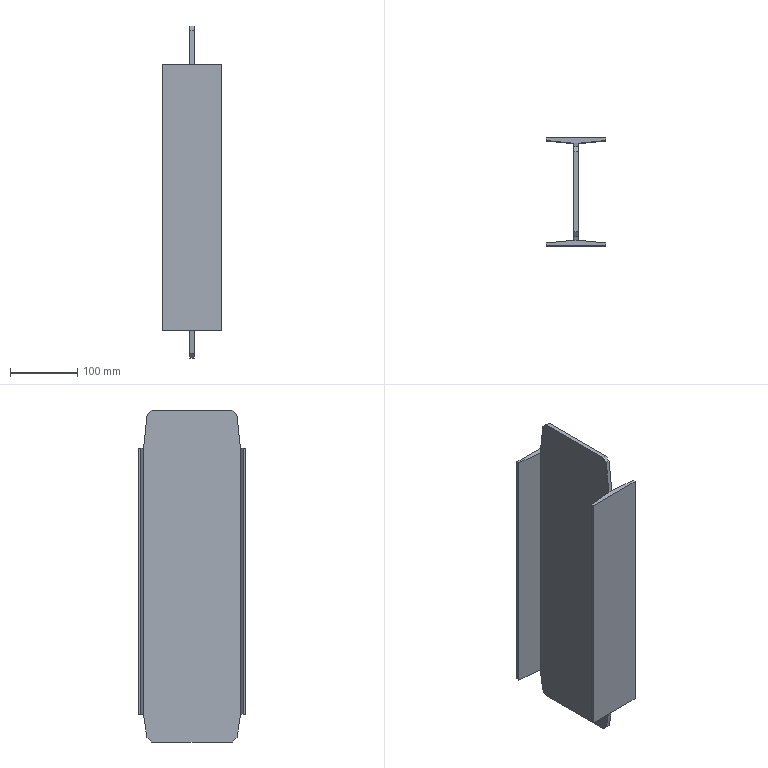Part | SolidWorks | features Chamfer 1, Extrusion 1, ICE 1 | 1 solid | 26 faces | box 88 x 160 x 493 mm | volume 848530 mm3 | plane 26
STEP:
#1=CARTESIAN_POINT('',(44.,-80.,189.5));
#2=VERTEX_POINT('',#1);
#3=CARTESIAN_POINT('',(44.,-80.,-205.5));
#4=VERTEX_POINT('',#3);
#5=CARTESIAN_POINT('',(44.,-80.,246.5));
#6=DIRECTION('',(0.,0.,-1.));
#7=VECTOR('',#6,1000.);
#8=LINE('',#5,#7);
#9=EDGE_CURVE('',#2,#4,#8,.T.);
#10=ORIENTED_EDGE('',*,*,#9,.F.);
#11=CARTESIAN_POINT('',(-44.,-80.,189.5));
#12=VERTEX_POINT('',#11);
#13=CARTESIAN_POINT('',(-44.,-80.,189.5));
#14=DIRECTION('',(1.,0.,0.));
#15=VECTOR('',#14,1000.);
#16=LINE('',#13,#15);
#17=EDGE_CURVE('',#12,#2,#16,.T.);
#18=ORIENTED_EDGE('',*,*,#17,.F.);
#19=CARTESIAN_POINT('',(-44.,-80.,-205.5));
#20=VERTEX_POINT('',#19);
#21=CARTESIAN_POINT('',(-44.,-80.,246.5));
#22=DIRECTION('',(0.,0.,-1.));
#23=VECTOR('',#22,1000.);
#24=LINE('',#21,#23);
#25=EDGE_CURVE('',#12,#20,#24,.T.);
#26=ORIENTED_EDGE('',*,*,#25,.T.);
#27=CARTESIAN_POINT('',(-44.,-80.,-205.5));
#28=DIRECTION('',(1.,0.,0.));
#29=VECTOR('',#28,1000.);
#30=LINE('',#27,#29);
#31=EDGE_CURVE('',#20,#4,#30,.T.);
#32=ORIENTED_EDGE('',*,*,#31,.T.);
#33=EDGE_LOOP('',(#10,#18,#26,#32));
#34=FACE_OUTER_BOUND('',#33,.T.);
#35=CARTESIAN_POINT('',(44.,-80.,246.5));
#36=DIRECTION('',(0.,1.,0.));
#37=DIRECTION('',(-1.,0.,0.));
#38=AXIS2_PLACEMENT_3D('',#35,#36,#37);
#39=PLANE('',#38);
#40=ADVANCED_FACE('',(#34),#39,.F.);
#41=CARTESIAN_POINT('',(44.,-76.,189.5));
#42=VERTEX_POINT('',#41);
#43=CARTESIAN_POINT('',(44.,-76.,-205.5));
#44=VERTEX_POINT('',#43);
#45=CARTESIAN_POINT('',(44.,-76.,246.5));
#46=DIRECTION('',(0.,0.,-1.));
#47=VECTOR('',#46,1000.);
#48=LINE('',#45,#47);
#49=EDGE_CURVE('',#42,#44,#48,.T.);
#50=ORIENTED_EDGE('',*,*,#49,.F.);
#51=CARTESIAN_POINT('',(44.,-72.,189.5));
#52=DIRECTION('',(0.,1.,0.));
#53=VECTOR('',#52,1000.);
#54=LINE('',#51,#53);
#55=EDGE_CURVE('',#2,#42,#54,.T.);
#56=ORIENTED_EDGE('',*,*,#55,.F.);
#57=ORIENTED_EDGE('',*,*,#9,.T.);
#58=CARTESIAN_POINT('',(44.,-72.,-205.5));
#59=DIRECTION('',(0.,-1.,0.));
#60=VECTOR('',#59,1000.);
#61=LINE('',#58,#60);
#62=EDGE_CURVE('',#44,#4,#61,.T.);
#63=ORIENTED_EDGE('',*,*,#62,.F.);
#64=EDGE_LOOP('',(#50,#56,#57,#63));
#65=FACE_OUTER_BOUND('',#64,.T.);
#66=CARTESIAN_POINT('',(44.,-80.,246.5));
#67=DIRECTION('',(-1.,0.,0.));
#68=DIRECTION('',(0.,-1.,0.));
#69=AXIS2_PLACEMENT_3D('',#66,#67,#68);
#70=PLANE('',#69);
#71=ADVANCED_FACE('',(#65),#70,.F.);
#72=CARTESIAN_POINT('',(3.,-72.,189.5));
#73=VERTEX_POINT('',#72);
#74=CARTESIAN_POINT('',(3.,-72.,-205.5));
#75=VERTEX_POINT('',#74);
#76=CARTESIAN_POINT('',(3.,-72.,246.5));
#77=DIRECTION('',(0.,0.,-1.));
#78=VECTOR('',#77,1000.);
#79=LINE('',#76,#78);
#80=EDGE_CURVE('',#73,#75,#79,.T.);
#81=ORIENTED_EDGE('',*,*,#80,.F.);
#82=CARTESIAN_POINT('',(44.,-76.,189.5));
#83=DIRECTION('',(0.9953,-0.0971,0.));
#84=VECTOR('',#83,1000.);
#85=LINE('',#82,#84);
#86=EDGE_CURVE('',#73,#42,#85,.T.);
#87=ORIENTED_EDGE('',*,*,#86,.T.);
#88=ORIENTED_EDGE('',*,*,#49,.T.);
#89=CARTESIAN_POINT('',(44.,-76.,-205.5));
#90=DIRECTION('',(-0.9953,0.0971,0.));
#91=VECTOR('',#90,1000.);
#92=LINE('',#89,#91);
#93=EDGE_CURVE('',#44,#75,#92,.T.);
#94=ORIENTED_EDGE('',*,*,#93,.T.);
#95=EDGE_LOOP('',(#81,#87,#88,#94));
#96=FACE_OUTER_BOUND('',#95,.T.);
#97=CARTESIAN_POINT('',(44.,-76.,246.5));
#98=DIRECTION('',(-0.0971,-0.9953,0.));
#99=DIRECTION('',(0.9953,-0.0971,0.));
#100=AXIS2_PLACEMENT_3D('',#97,#98,#99);
#101=PLANE('',#100);
#102=ADVANCED_FACE('',(#96),#101,.F.);
#103=CARTESIAN_POINT('',(3.,-59.257,246.5));
#104=VERTEX_POINT('',#103);
#105=CARTESIAN_POINT('',(3.,59.257,246.5));
#106=VERTEX_POINT('',#105);
#107=CARTESIAN_POINT('',(3.,72.,246.5));
#108=DIRECTION('',(0.,1.,0.));
#109=VECTOR('',#108,1000.);
#110=LINE('',#107,#109);
#111=EDGE_CURVE('',#104,#106,#110,.T.);
#112=ORIENTED_EDGE('',*,*,#111,.F.);
#113=CARTESIAN_POINT('',(3.,-66.628,240.533));
#114=VERTEX_POINT('',#113);
#115=CARTESIAN_POINT('',(3.,-59.257,246.5));
#116=DIRECTION('',(0.,-0.7772,-0.6292));
#117=VECTOR('',#116,1000.);
#118=LINE('',#115,#117);
#119=EDGE_CURVE('',#104,#114,#118,.T.);
#120=ORIENTED_EDGE('',*,*,#119,.T.);
#121=CARTESIAN_POINT('',(3.,-64.488,260.867));
#122=DIRECTION('',(0.,-0.1047,-0.9945));
#123=VECTOR('',#122,1000.);
#124=LINE('',#121,#123);
#125=EDGE_CURVE('',#114,#73,#124,.T.);
#126=ORIENTED_EDGE('',*,*,#125,.T.);
#127=ORIENTED_EDGE('',*,*,#80,.T.);
#128=CARTESIAN_POINT('',(3.,-67.029,-239.471));
#129=VERTEX_POINT('',#128);
#130=CARTESIAN_POINT('',(3.,-133.74,216.392));
#131=DIRECTION('',(0.,0.1448,-0.9895));
#132=VECTOR('',#131,1000.);
#133=LINE('',#130,#132);
#134=EDGE_CURVE('',#75,#129,#133,.T.);
#135=ORIENTED_EDGE('',*,*,#134,.T.);
#136=CARTESIAN_POINT('',(3.,-60.,-246.5));
#137=VERTEX_POINT('',#136);
#138=CARTESIAN_POINT('',(3.,-67.029,-239.471));
#139=DIRECTION('',(0.,0.7071,-0.7071));
#140=VECTOR('',#139,1000.);
#141=LINE('',#138,#140);
#142=EDGE_CURVE('',#129,#137,#141,.T.);
#143=ORIENTED_EDGE('',*,*,#142,.T.);
#144=CARTESIAN_POINT('',(3.,60.,-246.5));
#145=VERTEX_POINT('',#144);
#146=CARTESIAN_POINT('',(3.,72.,-246.5));
#147=DIRECTION('',(0.,1.,0.));
#148=VECTOR('',#147,1000.);
#149=LINE('',#146,#148);
#150=EDGE_CURVE('',#137,#145,#149,.T.);
#151=ORIENTED_EDGE('',*,*,#150,.T.);
#152=CARTESIAN_POINT('',(3.,67.029,-239.471));
#153=VERTEX_POINT('',#152);
#154=CARTESIAN_POINT('',(3.,67.029,-239.471));
#155=DIRECTION('',(0.,0.7071,0.7071));
#156=VECTOR('',#155,1000.);
#157=LINE('',#154,#156);
#158=EDGE_CURVE('',#145,#153,#157,.T.);
#159=ORIENTED_EDGE('',*,*,#158,.T.);
#160=CARTESIAN_POINT('',(3.,72.,-205.5));
#161=VERTEX_POINT('',#160);
#162=CARTESIAN_POINT('',(3.,136.759,237.023));
#163=DIRECTION('',(0.,0.1448,0.9895));
#164=VECTOR('',#163,1000.);
#165=LINE('',#162,#164);
#166=EDGE_CURVE('',#153,#161,#165,.T.);
#167=ORIENTED_EDGE('',*,*,#166,.T.);
#168=CARTESIAN_POINT('',(3.,72.,189.5));
#169=VERTEX_POINT('',#168);
#170=CARTESIAN_POINT('',(3.,72.,246.5));
#171=DIRECTION('',(0.,0.,-1.));
#172=VECTOR('',#171,1000.);
#173=LINE('',#170,#172);
#174=EDGE_CURVE('',#169,#161,#173,.T.);
#175=ORIENTED_EDGE('',*,*,#174,.F.);
#176=CARTESIAN_POINT('',(3.,66.628,240.533));
#177=VERTEX_POINT('',#176);
#178=CARTESIAN_POINT('',(3.,66.066,245.875));
#179=DIRECTION('',(0.,-0.1047,0.9945));
#180=VECTOR('',#179,1000.);
#181=LINE('',#178,#180);
#182=EDGE_CURVE('',#169,#177,#181,.T.);
#183=ORIENTED_EDGE('',*,*,#182,.T.);
#184=CARTESIAN_POINT('',(3.,59.257,246.5));
#185=DIRECTION('',(0.,-0.7772,0.6292));
#186=VECTOR('',#185,1000.);
#187=LINE('',#184,#186);
#188=EDGE_CURVE('',#177,#106,#187,.T.);
#189=ORIENTED_EDGE('',*,*,#188,.T.);
#190=EDGE_LOOP('',(#112,#120,#126,#127,#135,#143,#151,#159,#167,#175,#183,#189));
#191=FACE_OUTER_BOUND('',#190,.T.);
#192=CARTESIAN_POINT('',(3.,72.,246.5));
#193=DIRECTION('',(-1.,0.,0.));
#194=DIRECTION('',(0.,0.,1.));
#195=AXIS2_PLACEMENT_3D('',#192,#193,#194);
#196=PLANE('',#195);
#197=ADVANCED_FACE('',(#191),#196,.F.);
#198=ORIENTED_EDGE('',*,*,#174,.T.);
#199=CARTESIAN_POINT('',(44.,76.,-205.5));
#200=VERTEX_POINT('',#199);
#201=CARTESIAN_POINT('',(44.,76.,-205.5));
#202=DIRECTION('',(0.9953,0.0971,0.));
#203=VECTOR('',#202,1000.);
#204=LINE('',#201,#203);
#205=EDGE_CURVE('',#161,#200,#204,.T.);
#206=ORIENTED_EDGE('',*,*,#205,.T.);
#207=CARTESIAN_POINT('',(44.,76.,189.5));
#208=VERTEX_POINT('',#207);
#209=CARTESIAN_POINT('',(44.,76.,246.5));
#210=DIRECTION('',(0.,0.,-1.));
#211=VECTOR('',#210,1000.);
#212=LINE('',#209,#211);
#213=EDGE_CURVE('',#208,#200,#212,.T.);
#214=ORIENTED_EDGE('',*,*,#213,.F.);
#215=CARTESIAN_POINT('',(44.,76.,189.5));
#216=DIRECTION('',(-0.9953,-0.0971,0.));
#217=VECTOR('',#216,1000.);
#218=LINE('',#215,#217);
#219=EDGE_CURVE('',#208,#169,#218,.T.);
#220=ORIENTED_EDGE('',*,*,#219,.T.);
#221=EDGE_LOOP('',(#198,#206,#214,#220));
#222=FACE_OUTER_BOUND('',#221,.T.);
#223=CARTESIAN_POINT('',(44.,76.,246.5));
#224=DIRECTION('',(-0.0971,0.9953,0.));
#225=DIRECTION('',(-0.9953,-0.0971,0.));
#226=AXIS2_PLACEMENT_3D('',#223,#224,#225);
#227=PLANE('',#226);
#228=ADVANCED_FACE('',(#222),#227,.F.);
#229=ORIENTED_EDGE('',*,*,#213,.T.);
#230=CARTESIAN_POINT('',(44.,80.,-205.5));
#231=VERTEX_POINT('',#230);
#232=CARTESIAN_POINT('',(44.,72.,-205.5));
#233=DIRECTION('',(0.,-1.,0.));
#234=VECTOR('',#233,1000.);
#235=LINE('',#232,#234);
#236=EDGE_CURVE('',#231,#200,#235,.T.);
#237=ORIENTED_EDGE('',*,*,#236,.F.);
#238=CARTESIAN_POINT('',(44.,80.,189.5));
#239=VERTEX_POINT('',#238);
#240=CARTESIAN_POINT('',(44.,80.,246.5));
#241=DIRECTION('',(0.,0.,-1.));
#242=VECTOR('',#241,1000.);
#243=LINE('',#240,#242);
#244=EDGE_CURVE('',#239,#231,#243,.T.);
#245=ORIENTED_EDGE('',*,*,#244,.F.);
#246=CARTESIAN_POINT('',(44.,72.,189.5));
#247=DIRECTION('',(0.,1.,0.));
#248=VECTOR('',#247,1000.);
#249=LINE('',#246,#248);
#250=EDGE_CURVE('',#208,#239,#249,.T.);
#251=ORIENTED_EDGE('',*,*,#250,.F.);
#252=EDGE_LOOP('',(#229,#237,#245,#251));
#253=FACE_OUTER_BOUND('',#252,.T.);
#254=CARTESIAN_POINT('',(44.,80.,246.5));
#255=DIRECTION('',(-1.,0.,0.));
#256=DIRECTION('',(0.,-1.,0.));
#257=AXIS2_PLACEMENT_3D('',#254,#255,#256);
#258=PLANE('',#257);
#259=ADVANCED_FACE('',(#253),#258,.F.);
#260=ORIENTED_EDGE('',*,*,#244,.T.);
#261=CARTESIAN_POINT('',(-44.,80.,-205.5));
#262=VERTEX_POINT('',#261);
#263=CARTESIAN_POINT('',(-44.,80.,-205.5));
#264=DIRECTION('',(1.,0.,0.));
#265=VECTOR('',#264,1000.);
#266=LINE('',#263,#265);
#267=EDGE_CURVE('',#262,#231,#266,.T.);
#268=ORIENTED_EDGE('',*,*,#267,.F.);
#269=CARTESIAN_POINT('',(-44.,80.,189.5));
#270=VERTEX_POINT('',#269);
#271=CARTESIAN_POINT('',(-44.,80.,246.5));
#272=DIRECTION('',(0.,0.,-1.));
#273=VECTOR('',#272,1000.);
#274=LINE('',#271,#273);
#275=EDGE_CURVE('',#270,#262,#274,.T.);
#276=ORIENTED_EDGE('',*,*,#275,.F.);
#277=CARTESIAN_POINT('',(-44.,80.,189.5));
#278=DIRECTION('',(1.,0.,0.));
#279=VECTOR('',#278,1000.);
#280=LINE('',#277,#279);
#281=EDGE_CURVE('',#270,#239,#280,.T.);
#282=ORIENTED_EDGE('',*,*,#281,.T.);
#283=EDGE_LOOP('',(#260,#268,#276,#282));
#284=FACE_OUTER_BOUND('',#283,.T.);
#285=CARTESIAN_POINT('',(44.,80.,246.5));
#286=DIRECTION('',(0.,-1.,0.));
#287=DIRECTION('',(1.,0.,0.));
#288=AXIS2_PLACEMENT_3D('',#285,#286,#287);
#289=PLANE('',#288);
#290=ADVANCED_FACE('',(#284),#289,.F.);
#291=ORIENTED_EDGE('',*,*,#275,.T.);
#292=CARTESIAN_POINT('',(-44.,76.,-205.5));
#293=VERTEX_POINT('',#292);
#294=CARTESIAN_POINT('',(-44.,72.,-205.5));
#295=DIRECTION('',(0.,-1.,0.));
#296=VECTOR('',#295,1000.);
#297=LINE('',#294,#296);
#298=EDGE_CURVE('',#262,#293,#297,.T.);
#299=ORIENTED_EDGE('',*,*,#298,.T.);
#300=CARTESIAN_POINT('',(-44.,76.,189.5));
#301=VERTEX_POINT('',#300);
#302=CARTESIAN_POINT('',(-44.,76.,246.5));
#303=DIRECTION('',(0.,0.,-1.));
#304=VECTOR('',#303,1000.);
#305=LINE('',#302,#304);
#306=EDGE_CURVE('',#301,#293,#305,.T.);
#307=ORIENTED_EDGE('',*,*,#306,.F.);
#308=CARTESIAN_POINT('',(-44.,72.,189.5));
#309=DIRECTION('',(0.,1.,0.));
#310=VECTOR('',#309,1000.);
#311=LINE('',#308,#310);
#312=EDGE_CURVE('',#301,#270,#311,.T.);
#313=ORIENTED_EDGE('',*,*,#312,.T.);
#314=EDGE_LOOP('',(#291,#299,#307,#313));
#315=FACE_OUTER_BOUND('',#314,.T.);
#316=CARTESIAN_POINT('',(-44.,80.,246.5));
#317=DIRECTION('',(1.,0.,0.));
#318=DIRECTION('',(0.,1.,0.));
#319=AXIS2_PLACEMENT_3D('',#316,#317,#318);
#320=PLANE('',#319);
#321=ADVANCED_FACE('',(#315),#320,.F.);
#322=ORIENTED_EDGE('',*,*,#306,.T.);
#323=CARTESIAN_POINT('',(-3.,72.,-205.5));
#324=VERTEX_POINT('',#323);
#325=CARTESIAN_POINT('',(-44.,76.,-205.5));
#326=DIRECTION('',(0.9953,-0.0971,0.));
#327=VECTOR('',#326,1000.);
#328=LINE('',#325,#327);
#329=EDGE_CURVE('',#293,#324,#328,.T.);
#330=ORIENTED_EDGE('',*,*,#329,.T.);
#331=CARTESIAN_POINT('',(-3.,72.,189.5));
#332=VERTEX_POINT('',#331);
#333=CARTESIAN_POINT('',(-3.,72.,246.5));
#334=DIRECTION('',(0.,0.,-1.));
#335=VECTOR('',#334,1000.);
#336=LINE('',#333,#335);
#337=EDGE_CURVE('',#332,#324,#336,.T.);
#338=ORIENTED_EDGE('',*,*,#337,.F.);
#339=CARTESIAN_POINT('',(-44.,76.,189.5));
#340=DIRECTION('',(-0.9953,0.0971,0.));
#341=VECTOR('',#340,1000.);
#342=LINE('',#339,#341);
#343=EDGE_CURVE('',#332,#301,#342,.T.);
#344=ORIENTED_EDGE('',*,*,#343,.T.);
#345=EDGE_LOOP('',(#322,#330,#338,#344));
#346=FACE_OUTER_BOUND('',#345,.T.);
#347=CARTESIAN_POINT('',(-44.,76.,246.5));
#348=DIRECTION('',(0.0971,0.9953,0.));
#349=DIRECTION('',(-0.9953,0.0971,0.));
#350=AXIS2_PLACEMENT_3D('',#347,#348,#349);
#351=PLANE('',#350);
#352=ADVANCED_FACE('',(#346),#351,.F.);
#353=CARTESIAN_POINT('',(-3.,-72.,189.5));
#354=VERTEX_POINT('',#353);
#355=CARTESIAN_POINT('',(-3.,-66.628,240.533));
#356=VERTEX_POINT('',#355);
#357=CARTESIAN_POINT('',(-3.,-64.488,260.867));
#358=DIRECTION('',(0.,0.1047,0.9945));
#359=VECTOR('',#358,1000.);
#360=LINE('',#357,#359);
#361=EDGE_CURVE('',#354,#356,#360,.T.);
#362=ORIENTED_EDGE('',*,*,#361,.T.);
#363=CARTESIAN_POINT('',(-3.,-59.257,246.5));
#364=VERTEX_POINT('',#363);
#365=CARTESIAN_POINT('',(-3.,-59.257,246.5));
#366=DIRECTION('',(0.,0.7772,0.6292));
#367=VECTOR('',#366,1000.);
#368=LINE('',#365,#367);
#369=EDGE_CURVE('',#356,#364,#368,.T.);
#370=ORIENTED_EDGE('',*,*,#369,.T.);
#371=CARTESIAN_POINT('',(-3.,59.257,246.5));
#372=VERTEX_POINT('',#371);
#373=CARTESIAN_POINT('',(-3.,72.,246.5));
#374=DIRECTION('',(0.,-1.,0.));
#375=VECTOR('',#374,1000.);
#376=LINE('',#373,#375);
#377=EDGE_CURVE('',#372,#364,#376,.T.);
#378=ORIENTED_EDGE('',*,*,#377,.F.);
#379=CARTESIAN_POINT('',(-3.,66.628,240.533));
#380=VERTEX_POINT('',#379);
#381=CARTESIAN_POINT('',(-3.,59.257,246.5));
#382=DIRECTION('',(0.,0.7772,-0.6292));
#383=VECTOR('',#382,1000.);
#384=LINE('',#381,#383);
#385=EDGE_CURVE('',#372,#380,#384,.T.);
#386=ORIENTED_EDGE('',*,*,#385,.T.);
#387=CARTESIAN_POINT('',(-3.,66.066,245.875));
#388=DIRECTION('',(0.,0.1047,-0.9945));
#389=VECTOR('',#388,1000.);
#390=LINE('',#387,#389);
#391=EDGE_CURVE('',#380,#332,#390,.T.);
#392=ORIENTED_EDGE('',*,*,#391,.T.);
#393=ORIENTED_EDGE('',*,*,#337,.T.);
#394=CARTESIAN_POINT('',(-3.,67.029,-239.471));
#395=VERTEX_POINT('',#394);
#396=CARTESIAN_POINT('',(-3.,136.759,237.023));
#397=DIRECTION('',(0.,-0.1448,-0.9895));
#398=VECTOR('',#397,1000.);
#399=LINE('',#396,#398);
#400=EDGE_CURVE('',#324,#395,#399,.T.);
#401=ORIENTED_EDGE('',*,*,#400,.T.);
#402=CARTESIAN_POINT('',(-3.,60.,-246.5));
#403=VERTEX_POINT('',#402);
#404=CARTESIAN_POINT('',(-3.,67.029,-239.471));
#405=DIRECTION('',(0.,-0.7071,-0.7071));
#406=VECTOR('',#405,1000.);
#407=LINE('',#404,#406);
#408=EDGE_CURVE('',#395,#403,#407,.T.);
#409=ORIENTED_EDGE('',*,*,#408,.T.);
#410=CARTESIAN_POINT('',(-3.,-60.,-246.5));
#411=VERTEX_POINT('',#410);
#412=CARTESIAN_POINT('',(-3.,72.,-246.5));
#413=DIRECTION('',(0.,-1.,0.));
#414=VECTOR('',#413,1000.);
#415=LINE('',#412,#414);
#416=EDGE_CURVE('',#403,#411,#415,.T.);
#417=ORIENTED_EDGE('',*,*,#416,.T.);
#418=CARTESIAN_POINT('',(-3.,-67.029,-239.471));
#419=VERTEX_POINT('',#418);
#420=CARTESIAN_POINT('',(-3.,-67.029,-239.471));
#421=DIRECTION('',(0.,-0.7071,0.7071));
#422=VECTOR('',#421,1000.);
#423=LINE('',#420,#422);
#424=EDGE_CURVE('',#411,#419,#423,.T.);
#425=ORIENTED_EDGE('',*,*,#424,.T.);
#426=CARTESIAN_POINT('',(-3.,-72.,-205.5));
#427=VERTEX_POINT('',#426);
#428=CARTESIAN_POINT('',(-3.,-133.74,216.392));
#429=DIRECTION('',(0.,-0.1448,0.9895));
#430=VECTOR('',#429,1000.);
#431=LINE('',#428,#430);
#432=EDGE_CURVE('',#419,#427,#431,.T.);
#433=ORIENTED_EDGE('',*,*,#432,.T.);
#434=CARTESIAN_POINT('',(-3.,-72.,246.5));
#435=DIRECTION('',(0.,0.,-1.));
#436=VECTOR('',#435,1000.);
#437=LINE('',#434,#436);
#438=EDGE_CURVE('',#354,#427,#437,.T.);
#439=ORIENTED_EDGE('',*,*,#438,.F.);
#440=EDGE_LOOP('',(#362,#370,#378,#386,#392,#393,#401,#409,#417,#425,#433,#439));
#441=FACE_OUTER_BOUND('',#440,.T.);
#442=CARTESIAN_POINT('',(-3.,72.,246.5));
#443=DIRECTION('',(1.,0.,0.));
#444=DIRECTION('',(0.,0.,-1.));
#445=AXIS2_PLACEMENT_3D('',#442,#443,#444);
#446=PLANE('',#445);
#447=ADVANCED_FACE('',(#441),#446,.F.);
#448=CARTESIAN_POINT('',(-44.,-76.,189.5));
#449=VERTEX_POINT('',#448);
#450=CARTESIAN_POINT('',(-44.,-76.,-205.5));
#451=VERTEX_POINT('',#450);
#452=CARTESIAN_POINT('',(-44.,-76.,246.5));
#453=DIRECTION('',(0.,0.,-1.));
#454=VECTOR('',#453,1000.);
#455=LINE('',#452,#454);
#456=EDGE_CURVE('',#449,#451,#455,.T.);
#457=ORIENTED_EDGE('',*,*,#456,.F.);
#458=CARTESIAN_POINT('',(-44.,-76.,189.5));
#459=DIRECTION('',(0.9953,0.0971,0.));
#460=VECTOR('',#459,1000.);
#461=LINE('',#458,#460);
#462=EDGE_CURVE('',#449,#354,#461,.T.);
#463=ORIENTED_EDGE('',*,*,#462,.T.);
#464=ORIENTED_EDGE('',*,*,#438,.T.);
#465=CARTESIAN_POINT('',(-44.,-76.,-205.5));
#466=DIRECTION('',(-0.9953,-0.0971,0.));
#467=VECTOR('',#466,1000.);
#468=LINE('',#465,#467);
#469=EDGE_CURVE('',#427,#451,#468,.T.);
#470=ORIENTED_EDGE('',*,*,#469,.T.);
#471=EDGE_LOOP('',(#457,#463,#464,#470));
#472=FACE_OUTER_BOUND('',#471,.T.);
#473=CARTESIAN_POINT('',(-44.,-76.,246.5));
#474=DIRECTION('',(0.0971,-0.9953,0.));
#475=DIRECTION('',(0.9953,0.0971,0.));
#476=AXIS2_PLACEMENT_3D('',#473,#474,#475);
#477=PLANE('',#476);
#478=ADVANCED_FACE('',(#472),#477,.F.);
#479=ORIENTED_EDGE('',*,*,#25,.F.);
#480=CARTESIAN_POINT('',(-44.,-72.,189.5));
#481=DIRECTION('',(0.,1.,0.));
#482=VECTOR('',#481,1000.);
#483=LINE('',#480,#482);
#484=EDGE_CURVE('',#12,#449,#483,.T.);
#485=ORIENTED_EDGE('',*,*,#484,.T.);
#486=ORIENTED_EDGE('',*,*,#456,.T.);
#487=CARTESIAN_POINT('',(-44.,-72.,-205.5));
#488=DIRECTION('',(0.,-1.,0.));
#489=VECTOR('',#488,1000.);
#490=LINE('',#487,#489);
#491=EDGE_CURVE('',#451,#20,#490,.T.);
#492=ORIENTED_EDGE('',*,*,#491,.T.);
#493=EDGE_LOOP('',(#479,#485,#486,#492));
#494=FACE_OUTER_BOUND('',#493,.T.);
#495=CARTESIAN_POINT('',(-44.,-80.,246.5));
#496=DIRECTION('',(1.,0.,0.));
#497=DIRECTION('',(0.,1.,0.));
#498=AXIS2_PLACEMENT_3D('',#495,#496,#497);
#499=PLANE('',#498);
#500=ADVANCED_FACE('',(#494),#499,.F.);
#501=ORIENTED_EDGE('',*,*,#377,.T.);
#502=CARTESIAN_POINT('',(0.,-59.257,246.5));
#503=DIRECTION('',(1.,0.,0.));
#504=VECTOR('',#503,1000.);
#505=LINE('',#502,#504);
#506=EDGE_CURVE('',#364,#104,#505,.T.);
#507=ORIENTED_EDGE('',*,*,#506,.T.);
#508=ORIENTED_EDGE('',*,*,#111,.T.);
#509=CARTESIAN_POINT('',(0.,59.257,246.5));
#510=DIRECTION('',(-1.,0.,0.));
#511=VECTOR('',#510,1000.);
#512=LINE('',#509,#511);
#513=EDGE_CURVE('',#106,#372,#512,.T.);
#514=ORIENTED_EDGE('',*,*,#513,.T.);
#515=EDGE_LOOP('',(#501,#507,#508,#514));
#516=FACE_OUTER_BOUND('',#515,.T.);
#517=CARTESIAN_POINT('',(0.,0.,246.5));
#518=DIRECTION('',(0.,0.,-1.));
#519=DIRECTION('',(-1.,0.,0.));
#520=AXIS2_PLACEMENT_3D('',#517,#518,#519);
#521=PLANE('',#520);
#522=ADVANCED_FACE('',(#516),#521,.F.);
#523=ORIENTED_EDGE('',*,*,#150,.F.);
#524=CARTESIAN_POINT('',(-3.,-60.,-246.5));
#525=DIRECTION('',(-1.,0.,0.));
#526=VECTOR('',#525,1000.);
#527=LINE('',#524,#526);
#528=EDGE_CURVE('',#137,#411,#527,.T.);
#529=ORIENTED_EDGE('',*,*,#528,.T.);
#530=ORIENTED_EDGE('',*,*,#416,.F.);
#531=CARTESIAN_POINT('',(3.,60.,-246.5));
#532=DIRECTION('',(1.,0.,0.));
#533=VECTOR('',#532,1000.);
#534=LINE('',#531,#533);
#535=EDGE_CURVE('',#403,#145,#534,.T.);
#536=ORIENTED_EDGE('',*,*,#535,.T.);
#537=EDGE_LOOP('',(#523,#529,#530,#536));
#538=FACE_OUTER_BOUND('',#537,.T.);
#539=CARTESIAN_POINT('',(0.,0.,-246.5));
#540=DIRECTION('',(0.,0.,-1.));
#541=DIRECTION('',(-1.,0.,0.));
#542=AXIS2_PLACEMENT_3D('',#539,#540,#541);
#543=PLANE('',#542);
#544=ADVANCED_FACE('',(#538),#543,.T.);
#545=CARTESIAN_POINT('',(-44.,72.,-205.5));
#546=DIRECTION('',(1.,0.,0.));
#547=VECTOR('',#546,1000.);
#548=LINE('',#545,#547);
#549=EDGE_CURVE('',#324,#161,#548,.T.);
#550=ORIENTED_EDGE('',*,*,#549,.F.);
#551=ORIENTED_EDGE('',*,*,#329,.F.);
#552=ORIENTED_EDGE('',*,*,#298,.F.);
#553=ORIENTED_EDGE('',*,*,#267,.T.);
#554=ORIENTED_EDGE('',*,*,#236,.T.);
#555=ORIENTED_EDGE('',*,*,#205,.F.);
#556=EDGE_LOOP('',(#550,#551,#552,#553,#554,#555));
#557=FACE_OUTER_BOUND('',#556,.T.);
#558=CARTESIAN_POINT('',(-44.,72.,-205.5));
#559=DIRECTION('',(0.,0.,1.));
#560=DIRECTION('',(0.,-1.,0.));
#561=AXIS2_PLACEMENT_3D('',#558,#559,#560);
#562=PLANE('',#561);
#563=ADVANCED_FACE('',(#557),#562,.F.);
#564=ORIENTED_EDGE('',*,*,#166,.F.);
#565=CARTESIAN_POINT('',(-3.,67.029,-239.471));
#566=DIRECTION('',(-1.,0.,0.));
#567=VECTOR('',#566,1000.);
#568=LINE('',#565,#567);
#569=EDGE_CURVE('',#153,#395,#568,.T.);
#570=ORIENTED_EDGE('',*,*,#569,.T.);
#571=ORIENTED_EDGE('',*,*,#400,.F.);
#572=ORIENTED_EDGE('',*,*,#549,.T.);
#573=EDGE_LOOP('',(#564,#570,#571,#572));
#574=FACE_OUTER_BOUND('',#573,.T.);
#575=CARTESIAN_POINT('',(-44.,66.,-246.5));
#576=DIRECTION('',(0.,-0.9895,0.1448));
#577=DIRECTION('',(0.,-0.1448,-0.9895));
#578=AXIS2_PLACEMENT_3D('',#575,#576,#577);
#579=PLANE('',#578);
#580=ADVANCED_FACE('',(#574),#579,.F.);
#581=ORIENTED_EDGE('',*,*,#62,.T.);
#582=ORIENTED_EDGE('',*,*,#31,.F.);
#583=ORIENTED_EDGE('',*,*,#491,.F.);
#584=ORIENTED_EDGE('',*,*,#469,.F.);
#585=CARTESIAN_POINT('',(-44.,-72.,-205.5));
#586=DIRECTION('',(1.,0.,0.));
#587=VECTOR('',#586,1000.);
#588=LINE('',#585,#587);
#589=EDGE_CURVE('',#427,#75,#588,.T.);
#590=ORIENTED_EDGE('',*,*,#589,.T.);
#591=ORIENTED_EDGE('',*,*,#93,.F.);
#592=EDGE_LOOP('',(#581,#582,#583,#584,#590,#591));
#593=FACE_OUTER_BOUND('',#592,.T.);
#594=CARTESIAN_POINT('',(-44.,-72.,-205.5));
#595=DIRECTION('',(0.,0.,1.));
#596=DIRECTION('',(0.,-1.,0.));
#597=AXIS2_PLACEMENT_3D('',#594,#595,#596);
#598=PLANE('',#597);
#599=ADVANCED_FACE('',(#593),#598,.F.);
#600=ORIENTED_EDGE('',*,*,#432,.F.);
#601=CARTESIAN_POINT('',(3.,-67.029,-239.471));
#602=DIRECTION('',(1.,0.,0.));
#603=VECTOR('',#602,1000.);
#604=LINE('',#601,#603);
#605=EDGE_CURVE('',#419,#129,#604,.T.);
#606=ORIENTED_EDGE('',*,*,#605,.T.);
#607=ORIENTED_EDGE('',*,*,#134,.F.);
#608=ORIENTED_EDGE('',*,*,#589,.F.);
#609=EDGE_LOOP('',(#600,#606,#607,#608));
#610=FACE_OUTER_BOUND('',#609,.T.);
#611=CARTESIAN_POINT('',(-44.,-66.,-246.5));
#612=DIRECTION('',(0.,0.9895,0.1448));
#613=DIRECTION('',(0.,-0.1448,0.9895));
#614=AXIS2_PLACEMENT_3D('',#611,#612,#613);
#615=PLANE('',#614);
#616=ADVANCED_FACE('',(#610),#615,.F.);
#617=ORIENTED_EDGE('',*,*,#250,.T.);
#618=ORIENTED_EDGE('',*,*,#281,.F.);
#619=ORIENTED_EDGE('',*,*,#312,.F.);
#620=ORIENTED_EDGE('',*,*,#343,.F.);
#621=CARTESIAN_POINT('',(-44.,72.,189.5));
#622=DIRECTION('',(1.,0.,0.));
#623=VECTOR('',#622,1000.);
#624=LINE('',#621,#623);
#625=EDGE_CURVE('',#332,#169,#624,.T.);
#626=ORIENTED_EDGE('',*,*,#625,.T.);
#627=ORIENTED_EDGE('',*,*,#219,.F.);
#628=EDGE_LOOP('',(#617,#618,#619,#620,#626,#627));
#629=FACE_OUTER_BOUND('',#628,.T.);
#630=CARTESIAN_POINT('',(-44.,72.,189.5));
#631=DIRECTION('',(0.,0.,-1.));
#632=DIRECTION('',(-1.,0.,0.));
#633=AXIS2_PLACEMENT_3D('',#630,#631,#632);
#634=PLANE('',#633);
#635=ADVANCED_FACE('',(#629),#634,.F.);
#636=ORIENTED_EDGE('',*,*,#391,.F.);
#637=CARTESIAN_POINT('',(-44.,66.628,240.533));
#638=DIRECTION('',(1.,0.,0.));
#639=VECTOR('',#638,1000.);
#640=LINE('',#637,#639);
#641=EDGE_CURVE('',#380,#177,#640,.T.);
#642=ORIENTED_EDGE('',*,*,#641,.T.);
#643=ORIENTED_EDGE('',*,*,#182,.F.);
#644=ORIENTED_EDGE('',*,*,#625,.F.);
#645=EDGE_LOOP('',(#636,#642,#643,#644));
#646=FACE_OUTER_BOUND('',#645,.T.);
#647=CARTESIAN_POINT('',(-44.,66.,246.5));
#648=DIRECTION('',(0.,-0.9945,-0.1047));
#649=DIRECTION('',(0.,0.1047,-0.9945));
#650=AXIS2_PLACEMENT_3D('',#647,#648,#649);
#651=PLANE('',#650);
#652=ADVANCED_FACE('',(#646),#651,.F.);
#653=CARTESIAN_POINT('',(-44.,-72.,189.5));
#654=DIRECTION('',(1.,0.,0.));
#655=VECTOR('',#654,1000.);
#656=LINE('',#653,#655);
#657=EDGE_CURVE('',#354,#73,#656,.T.);
#658=ORIENTED_EDGE('',*,*,#657,.F.);
#659=ORIENTED_EDGE('',*,*,#462,.F.);
#660=ORIENTED_EDGE('',*,*,#484,.F.);
#661=ORIENTED_EDGE('',*,*,#17,.T.);
#662=ORIENTED_EDGE('',*,*,#55,.T.);
#663=ORIENTED_EDGE('',*,*,#86,.F.);
#664=EDGE_LOOP('',(#658,#659,#660,#661,#662,#663));
#665=FACE_OUTER_BOUND('',#664,.T.);
#666=CARTESIAN_POINT('',(-44.,-72.,189.5));
#667=DIRECTION('',(0.,0.,-1.));
#668=DIRECTION('',(-1.,0.,0.));
#669=AXIS2_PLACEMENT_3D('',#666,#667,#668);
#670=PLANE('',#669);
#671=ADVANCED_FACE('',(#665),#670,.F.);
#672=ORIENTED_EDGE('',*,*,#125,.F.);
#673=CARTESIAN_POINT('',(-44.,-66.628,240.533));
#674=DIRECTION('',(-1.,0.,0.));
#675=VECTOR('',#674,1000.);
#676=LINE('',#673,#675);
#677=EDGE_CURVE('',#114,#356,#676,.T.);
#678=ORIENTED_EDGE('',*,*,#677,.T.);
#679=ORIENTED_EDGE('',*,*,#361,.F.);
#680=ORIENTED_EDGE('',*,*,#657,.T.);
#681=EDGE_LOOP('',(#672,#678,#679,#680));
#682=FACE_OUTER_BOUND('',#681,.T.);
#683=CARTESIAN_POINT('',(-44.,-66.,246.5));
#684=DIRECTION('',(0.,0.9945,-0.1047));
#685=DIRECTION('',(0.,0.1047,0.9945));
#686=AXIS2_PLACEMENT_3D('',#683,#684,#685);
#687=PLANE('',#686);
#688=ADVANCED_FACE('',(#682),#687,.F.);
#689=ORIENTED_EDGE('',*,*,#369,.F.);
#690=ORIENTED_EDGE('',*,*,#677,.F.);
#691=ORIENTED_EDGE('',*,*,#119,.F.);
#692=ORIENTED_EDGE('',*,*,#506,.F.);
#693=EDGE_LOOP('',(#689,#690,#691,#692));
#694=FACE_OUTER_BOUND('',#693,.T.);
#695=CARTESIAN_POINT('',(0.,-59.257,246.5));
#696=DIRECTION('',(0.,0.6292,-0.7772));
#697=DIRECTION('',(1.,0.,0.));
#698=AXIS2_PLACEMENT_3D('',#695,#696,#697);
#699=PLANE('',#698);
#700=ADVANCED_FACE('',(#694),#699,.F.);
#701=ORIENTED_EDGE('',*,*,#424,.F.);
#702=ORIENTED_EDGE('',*,*,#528,.F.);
#703=ORIENTED_EDGE('',*,*,#142,.F.);
#704=ORIENTED_EDGE('',*,*,#605,.F.);
#705=EDGE_LOOP('',(#701,#702,#703,#704));
#706=FACE_OUTER_BOUND('',#705,.T.);
#707=CARTESIAN_POINT('',(-44.,-67.029,-239.471));
#708=DIRECTION('',(0.,-0.7071,-0.7071));
#709=DIRECTION('',(-1.,0.,0.));
#710=AXIS2_PLACEMENT_3D('',#707,#708,#709);
#711=PLANE('',#710);
#712=ADVANCED_FACE('',(#706),#711,.T.);
#713=ORIENTED_EDGE('',*,*,#158,.F.);
#714=ORIENTED_EDGE('',*,*,#535,.F.);
#715=ORIENTED_EDGE('',*,*,#408,.F.);
#716=ORIENTED_EDGE('',*,*,#569,.F.);
#717=EDGE_LOOP('',(#713,#714,#715,#716));
#718=FACE_OUTER_BOUND('',#717,.T.);
#719=CARTESIAN_POINT('',(-44.,67.029,-239.471));
#720=DIRECTION('',(0.,0.7071,-0.7071));
#721=DIRECTION('',(1.,0.,0.));
#722=AXIS2_PLACEMENT_3D('',#719,#720,#721);
#723=PLANE('',#722);
#724=ADVANCED_FACE('',(#718),#723,.T.);
#725=ORIENTED_EDGE('',*,*,#188,.F.);
#726=ORIENTED_EDGE('',*,*,#641,.F.);
#727=ORIENTED_EDGE('',*,*,#385,.F.);
#728=ORIENTED_EDGE('',*,*,#513,.F.);
#729=EDGE_LOOP('',(#725,#726,#727,#728));
#730=FACE_OUTER_BOUND('',#729,.T.);
#731=CARTESIAN_POINT('',(0.,59.257,246.5));
#732=DIRECTION('',(0.,-0.6292,-0.7772));
#733=DIRECTION('',(-1.,0.,0.));
#734=AXIS2_PLACEMENT_3D('',#731,#732,#733);
#735=PLANE('',#734);
#736=ADVANCED_FACE('',(#730),#735,.F.);
#737=CLOSED_SHELL('',(#40,#71,#102,#197,#228,#259,#290,#321,#352,#447,#478,#500,#522,#544,#563,#580,#599,#616,#635,#652,#671,#688,#700,#712,#724,#736));
#738=MANIFOLD_SOLID_BREP('',#737);
#739=CARTESIAN_POINT('',(0.,0.,0.));
#740=DIRECTION('',(0.,0.,1.));
#741=DIRECTION('',(1.,0.,0.));
#742=AXIS2_PLACEMENT_3D('',#739,#740,#741);
#743=(LENGTH_UNIT()NAMED_UNIT(*)SI_UNIT(.MILLI.,.METRE.));
#744=UNCERTAINTY_MEASURE_WITH_UNIT(LENGTH_MEASURE(0.00001),#743,'','');
#745=(NAMED_UNIT(*)PLANE_ANGLE_UNIT()SI_UNIT($,.RADIAN.));
#746=(NAMED_UNIT(*)SI_UNIT($,.STERADIAN.)SOLID_ANGLE_UNIT());
#747=(GEOMETRIC_REPRESENTATION_CONTEXT(3)GLOBAL_UNCERTAINTY_ASSIGNED_CONTEXT((#744))GLOBAL_UNIT_ASSIGNED_CONTEXT((#743,#745,#746))REPRESENTATION_CONTEXT('',''));
#748=ADVANCED_BREP_SHAPE_REPRESENTATION('',(#738,#742),#747);